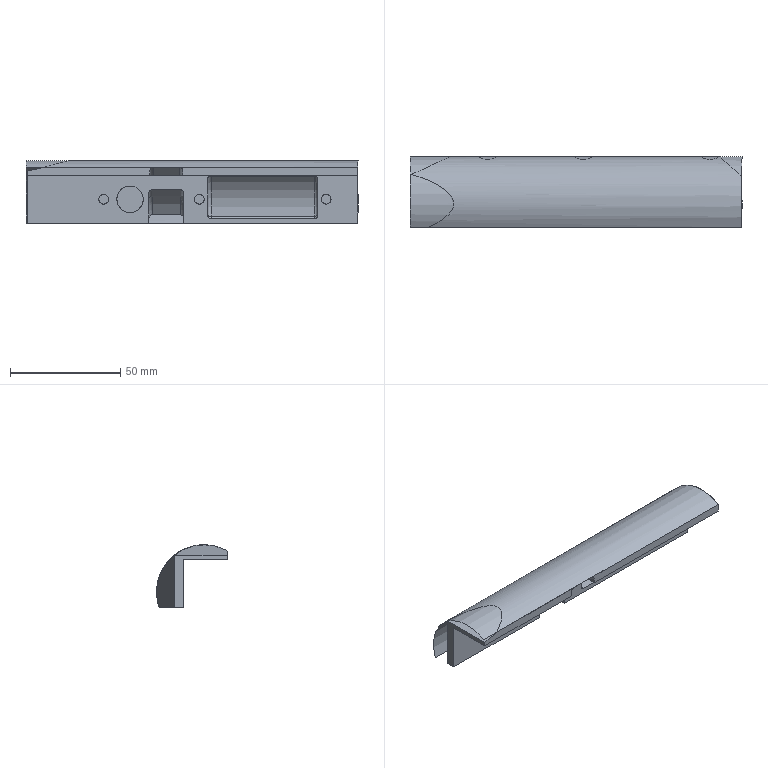NC program | Mastercam | posted with a generic post
Lines 32 to 1434 of 52802:
(10 FEM |TOOL - 9|DIA. OFF. - 9|LEN. - 9|TOOL DIA. - 10.)
N134 T9 M6
N136 G0 G54 G90 X-82.823 Y-24.256 C0. B0. S6500 M3
N138 G43 H9 Z20.
N140 Z1.
N142 G1 Z-16.25 F600.
N144 X-83.124 Y-23.448 Z-16.368 F4000.
N146 G3 X-83.642 Y-22.642 Z-16.5 I-2.109 J-.785
N148 G1 X-83.884 Y-22.278
N150 X-84.136 Y-21.786
N152 X-84.344 Y-21.317
N154 X-84.509 Y-20.881
N156 X-84.635 Y-20.477
N158 X-84.731 Y-20.104
N160 X-84.803 Y-19.761
N162 X-84.857 Y-19.444
N164 X-84.898 Y-19.15
N166 X-84.952 Y-18.629
N168 X-84.985 Y-18.155
N170 X-85.006 Y-17.715
N172 X-85.018 Y-17.3
N174 X-85.025 Y-16.902
N176 X-85.029 Y-16.516
N178 X-85.031 Y-16.138
N180 X-85.032 Y-15.766
N182 X-85.031 Y-15.397
N184 X-85.03 Y-15.031
N186 X-85.029 Y-14.667
N188 X-85.027 Y-14.303
N190 X-85.026 Y-13.94
N192 X-85.024 Y-13.577
N194 X-85.022 Y-13.215
N196 X-85.02 Y-12.852
N198 X-85.018 Y-12.49
N200 X-85.016 Y-12.127
N202 X-85.014 Y-11.765
N204 X-85.012 Y-11.402
N206 X-85.011 Y-11.04
N208 X-85.009 Y-10.677
N210 X-85.007 Y-10.314
N212 X-85.005 Y-9.951
N214 X-85.003 Y-9.588
N216 X-85.001 Y-9.226
N218 X-84.999 Y-8.863
N220 X-84.997 Y-8.5
N222 X-84.995 Y-8.137
N224 X-84.993 Y-7.774
N226 X-84.991 Y-7.41
N228 X-84.989 Y-7.047
N230 X-84.988 Y-6.684
N232 X-84.986 Y-6.321
N234 X-84.984 Y-5.958
N236 X-84.982 Y-5.594
N238 X-84.98 Y-5.231
N240 X-84.978 Y-4.867
N242 X-84.976 Y-4.504
N244 X-84.974 Y-4.14
N246 X-84.972 Y-3.777
N248 X-84.97 Y-3.413
N250 X-84.968 Y-3.05
N252 X-84.966 Y-2.686
N254 X-84.964 Y-2.322
N256 X-84.962 Y-1.958
N258 X-84.961 Y-1.595
N260 X-84.959 Y-1.231
N262 X-84.957 Y-.867
N264 X-84.955 Y-.503
N266 X-84.953 Y-.139
N268 X-84.951 Y.225
N270 X-84.949 Y.589
N272 X-84.947 Y.953
N274 X-84.945 Y1.317
N276 X-84.943 Y1.681
N278 X-84.941 Y2.045
N280 X-84.939 Y2.409
N282 X-84.937 Y2.773
N284 X-84.935 Y3.138
N286 X-84.934 Y3.502
N288 X-84.932 Y3.866
N290 X-84.93 Y4.23
N292 X-84.928 Y4.595
N294 X-84.926 Y4.959
N296 X-84.924 Y5.323
N298 X-84.922 Y5.688
N300 X-84.92 Y6.052
N302 X-84.918 Y6.417
N304 X-84.916 Y6.781
N306 X-84.914 Y7.146
N308 X-84.912 Y7.51
N310 X-84.91 Y7.875
N312 X-84.908 Y8.24
N314 X-84.906 Y8.604
N316 X-84.905 Y8.969
N318 X-84.903 Y9.333
N320 X-84.901 Y9.698
N322 X-84.899 Y10.063
N324 X-84.897 Y10.428
N326 X-84.895 Y10.792
N328 X-84.893 Y11.157
N330 X-84.891 Y11.522
N332 X-84.889 Y11.887
N334 X-84.887 Y12.252
N336 X-84.885 Y12.617
N338 X-84.883 Y12.982
N340 X-84.881 Y13.346
N342 X-84.879 Y13.711
N344 X-84.877 Y14.076
N346 X-84.876 Y14.441
N348 X-84.874 Y14.806
N350 X-84.872 Y15.171
N352 X-84.87 Y15.537
N354 X-84.868 Y15.902
N356 X-84.866 Y16.267
N358 X-84.864 Y16.632
N360 X-84.862 Y16.997
N362 X-84.86 Y17.374
N364 X-84.843 Y17.804
N366 X-84.784 Y18.268
N368 X-84.68 Y18.729
N370 X-84.532 Y19.182
N372 X-84.344 Y19.62
N374 X-84.12 Y20.036
N376 X-83.865 Y20.427
N378 X-83.585 Y20.789
N380 X-83.287 Y21.121
N382 X-82.974 Y21.423
N384 X-82.653 Y21.695
N386 X-82.326 Y21.938
N388 X-81.999 Y22.154
N390 X-81.672 Y22.346
N392 X-81.349 Y22.515
N394 X-81.032 Y22.664
N396 X-80.721 Y22.794
N398 X-80.417 Y22.909
N400 X-80.12 Y23.009
N402 X-79.831 Y23.096
N404 X-79.55 Y23.173
N406 X-79.019 Y23.298
N408 X-78.513 Y23.395
N410 X-78.027 Y23.471
N412 X-77.561 Y23.53
N414 X-77.111 Y23.577
N416 X-76.675 Y23.614
N418 X-76.251 Y23.642
N420 X-75.838 Y23.665
N422 X-75.433 Y23.683
N424 X-75.035 Y23.697
N426 X-74.642 Y23.707
N428 X-74.255 Y23.715
N430 X-73.872 Y23.722
N432 X-73.491 Y23.726
N434 X-73.114 Y23.729
N436 X-72.739 Y23.732
N438 X-72.366 Y23.733
N440 X-71.994
N442 X-71.623
N444 X-71.254
N446 X-70.885 Y23.732
N448 X-70.517 Y23.731
N450 X-70.149 Y23.73
N452 X-69.782 Y23.728
N454 X-69.415 Y23.727
N456 X-69.048 Y23.725
N458 X-68.682 Y23.723
N460 X-68.315 Y23.722
N462 X-67.948 Y23.72
N464 X-67.582 Y23.718
N466 X-67.216 Y23.716
N468 X-66.849 Y23.714
N470 X-66.483 Y23.712
N472 X-66.116 Y23.71
N474 X-65.75 Y23.708
N476 X-65.384 Y23.707
N478 X-65.017 Y23.705
N480 X-64.651 Y23.703
N482 X-64.285 Y23.701
N484 X-63.918 Y23.699
N486 X-63.552 Y23.697
N488 X-63.186 Y23.695
N490 X-62.819 Y23.693
N492 X-62.453 Y23.691
N494 X-62.086 Y23.689
N496 X-61.72 Y23.687
N498 X-61.354 Y23.685
N500 X-60.987 Y23.683
N502 X-60.621 Y23.681
N504 X-60.254 Y23.679
N506 X-59.888 Y23.677
N508 X-59.521 Y23.676
N510 X-59.155 Y23.674
N512 X-58.788 Y23.672
N514 X-58.422 Y23.67
N516 X-58.055 Y23.668
N518 X-57.689 Y23.666
N520 X-57.322 Y23.664
N522 X-56.956 Y23.662
N524 X-56.589 Y23.66
N526 X-56.221 Y23.658
N528 X-55.853 Y23.657
N530 X-55.485 Y23.656
N532 X-55.116 Y23.655
N534 X-54.747 Y23.654
N536 X-54.378
N538 X-54.008 Y23.653
N540 X-53.638
N542 X-53.269 Y23.652
N544 X-52.899
N546 X-52.529
N548 X-52.158 Y23.651
N550 X-51.788
N552 X-51.418
N554 X-51.048
N556 X-50.677
N558 X-50.307
N560 X-49.936 Y23.65
N562 X-49.566
N564 X-49.195
N566 X-48.825
N568 X-48.454
N570 X-48.084
N572 X-47.713
N574 X-47.343
N576 X-46.972
N578 X-46.602
N580 X-46.231
N582 X-45.861
N584 X-45.49
N586 X-45.119
N588 X-44.749
N590 X-44.378
N592 X-44.008
N594 X-43.637
N596 X-43.266
N598 X-42.896
N600 X-42.525
N602 X-42.155
N604 X-41.784
N606 X-41.413
N608 X-41.043
N610 X-40.672
N612 X-40.302
N614 X-39.931
N616 X-39.56
N618 X-39.19
N620 X-38.819
N622 X-38.449
N624 X-38.078
N626 X-37.707
N628 X-37.337
N630 X-36.966
N632 X-36.596
N634 X-36.225
N636 X-35.854
N638 X-35.484
N640 X-35.113
N642 X-34.743
N644 X-34.372
N646 X-34.001
N648 X-33.631
N650 X-33.26
N652 X-32.89
N654 X-32.519
N656 X-32.148
N658 X-31.778
N660 X-31.407
N662 X-31.037
N664 X-30.666
N666 X-30.295
N668 X-29.925
N670 X-29.554
N672 X-29.184
N674 X-28.813
N676 X-28.442
N678 X-28.072
N680 X-27.701
N682 X-27.331
N684 X-26.96
N686 X-26.589
N688 X-26.219
N690 X-25.848
N692 X-25.477
N694 X-25.107
N696 X-24.736
N698 X-24.366
N700 X-23.995
N702 X-23.624
N704 X-23.254
N706 X-22.883
N708 X-22.513
N710 X-22.142
N712 X-21.771
N714 X-21.401
N716 X-21.03
N718 X-20.66
N720 X-20.289
N722 X-19.918
N724 X-19.548
N726 X-19.177
N728 X-18.807
N730 X-18.436
N732 X-18.065
N734 X-17.695
N736 X-17.324
N738 X-16.954
N740 X-16.583
N742 X-16.212
N744 X-15.842
N746 X-15.471
N748 X-15.101
N750 X-14.73
N752 X-14.359
N754 X-13.989
N756 X-13.618
N758 X-13.248
N760 X-12.877
N762 X-12.506
N764 X-12.136
N766 X-11.765
N768 X-11.395
N770 X-11.024
N772 X-10.653
N774 X-10.283
N776 X-9.912
N778 X-9.542
N780 X-9.171
N782 X-8.8
N784 X-8.43
N786 X-8.059
N788 X-7.689
N790 X-7.318
N792 X-6.947
N794 X-6.577
N796 X-6.206
N798 X-5.835
N800 X-5.465
N802 X-5.094
N804 X-4.724
N806 X-4.353
N808 X-3.982
N810 X-3.612
N812 X-3.241
N814 X-2.871
N816 X-2.5
N818 X-2.129
N820 X-1.759
N822 X-1.388
N824 X-1.018
N826 X-.647
N828 X-.276
N830 X.094
N832 X.465
N834 X.835
N836 X1.206
N838 X1.577
N840 X1.947
N842 X2.318
N844 X2.688
N846 X3.059
N848 X3.43
N850 X3.8
N852 X4.171
N854 X4.541
N856 X4.912
N858 X5.283
N860 X5.653
N862 X6.024
N864 X6.394
N866 X6.765
N868 X7.136
N870 X7.506
N872 X7.877
N874 X8.247
N876 X8.618
N878 X8.989
N880 X9.359
N882 X9.73
N884 X10.1
N886 X10.471
N888 X10.842
N890 X11.212
N892 X11.583
N894 X11.953
N896 X12.324
N898 X12.695
N900 X13.065
N902 X13.436
N904 X13.807
N906 X14.177
N908 X14.548
N910 X14.918
N912 X15.289
N914 X15.66
N916 X16.03
N918 X16.401
N920 X16.771
N922 X17.142
N924 X17.513
N926 X17.883
N928 X18.254
N930 X18.624
N932 X18.995
N934 X19.366
N936 X19.736
N938 X20.107
N940 X20.477
N942 X20.848
N944 X21.219
N946 X21.589
N948 X21.96
N950 X22.33
N952 X22.701
N954 X23.072
N956 X23.442
N958 X23.813
N960 X24.183
N962 X24.554
N964 X24.925
N966 X25.295
N968 X25.666
N970 X26.036
N972 X26.407
N974 X26.778
N976 X27.148
N978 X27.519
N980 X27.889
N982 X28.26
N984 X28.631
N986 X29.001
N988 X29.372
N990 X29.742
N992 X30.113
N994 X30.484
N996 X30.854
N998 X31.225
N1000 X31.596
N1002 X31.966
N1004 X32.337
N1006 X32.707
N1008 X33.078
N1010 X33.449
N1012 X33.819
N1014 X34.19
N1016 X34.56
N1018 X34.931
N1020 X35.302
N1022 X35.672
N1024 X36.043
N1026 X36.413
N1028 X36.784
N1030 X37.155
N1032 X37.525
N1034 X37.896
N1036 X38.266
N1038 X38.637
N1040 X39.008
N1042 X39.378
N1044 X39.749
N1046 X40.119
N1048 X40.49
N1050 X40.861
N1052 X41.231
N1054 X41.602
N1056 X41.972
N1058 X42.343
N1060 X42.714
N1062 X43.084
N1064 X43.455
N1066 X43.825
N1068 X44.196
N1070 X44.567
N1072 X44.937
N1074 X45.308
N1076 X45.678
N1078 X46.049
N1080 X46.42
N1082 X46.79
N1084 X47.161
N1086 X47.531
N1088 X47.902
N1090 X48.273
N1092 X48.643
N1094 X49.014
N1096 X49.384
N1098 X49.755
N1100 X50.126
N1102 X50.496
N1104 X50.867
N1106 X51.238
N1108 X51.608
N1110 X51.979
N1112 X52.349
N1114 X52.72
N1116 X53.091
N1118 X53.461
N1120 X53.832
N1122 X54.202
N1124 X54.573
N1126 X54.944
N1128 X55.314
N1130 X55.685
N1132 X56.055
N1134 X56.426
N1136 X56.797
N1138 X57.167
N1140 X57.538
N1142 X57.908
N1144 X58.279
N1146 X58.65
N1148 X59.02
N1150 X59.391
N1152 X59.761
N1154 X60.132
N1156 X60.503
N1158 X60.873
N1160 X61.244
N1162 X61.614
N1164 X61.985
N1166 X62.356
N1168 X62.726
N1170 X63.097
N1172 X63.467
N1174 X63.838
N1176 X64.209
N1178 X64.579
N1180 X64.95
N1182 X65.32
N1184 X65.691
N1186 X66.062
N1188 X66.432
N1190 X66.803
N1192 X67.173
N1194 X67.544
N1196 X67.915
N1198 X68.285
N1200 X68.656
N1202 X69.026
N1204 X69.397
N1206 X69.768
N1208 X70.138
N1210 X70.509
N1212 X70.88
N1214 X71.25
N1216 X71.621
N1218 X71.991
N1220 X72.362
N1222 X72.733
N1224 X73.103
N1226 X73.474
N1228 X73.844
N1230 X74.215
N1232 X74.586
N1234 X74.956
N1236 X75.327
N1238 X75.697
N1240 X76.068
N1242 X76.439
N1244 X76.809
N1246 X77.18
N1248 X77.55
N1250 X77.971 Y23.649
N1252 X78.348 Y23.632
N1254 X78.718 Y23.587
N1256 X79.092 Y23.512
N1258 X79.466 Y23.406
N1260 X79.836 Y23.27
N1262 X80.197 Y23.107
N1264 X80.546 Y22.919
N1266 X80.88 Y22.707
N1268 X81.198 Y22.476
N1270 X81.497 Y22.227
N1272 X81.777 Y21.965
N1274 X82.037 Y21.692
N1276 X82.277 Y21.41
N1278 X82.498 Y21.123
N1280 X82.701 Y20.832
N1282 X82.885 Y20.539
N1284 X83.053 Y20.247
N1286 X83.206 Y19.955
N1288 X83.344 Y19.665
N1290 X83.468 Y19.379
N1292 X83.581 Y19.096
N1294 X83.683 Y18.817
N1296 X83.774 Y18.542
N1298 X83.929 Y18.016
N1300 X84.056 Y17.507
N1302 X84.159 Y17.013
N1304 X84.244 Y16.535
N1306 X84.313 Y16.071
N1308 X84.37 Y15.62
N1310 X84.417 Y15.18
N1312 X84.456 Y14.75
N1314 X84.488 Y14.328
N1316 X84.514 Y13.914
N1318 X84.536 Y13.506
N1320 X84.555 Y13.104
N1322 X84.57 Y12.707
N1324 X84.583 Y12.314
N1326 X84.594 Y11.924
N1328 X84.603 Y11.537
N1330 X84.61 Y11.153
N1332 X84.617 Y10.771
N1334 X84.622 Y10.39
N1336 X84.626 Y10.012
N1338 X84.63 Y9.634
N1340 X84.633 Y9.258
N1342 X84.636 Y8.882
N1344 X84.638 Y8.507
N1346 X84.64 Y8.133
N1348 X84.642 Y7.759
N1350 X84.643 Y7.386
N1352 X84.644 Y7.013
N1354 X84.645 Y6.641
N1356 X84.646 Y6.269
N1358 Y5.897
N1360 X84.647 Y5.525
N1362 Y5.154
N1364 X84.648 Y4.783
N1366 Y4.411
N1368 Y4.04
N1370 X84.649 Y3.669
N1372 Y3.298
N1374 Y2.927
N1376 Y2.556
N1378 Y2.185
N1380 Y1.815
N1382 X84.65 Y1.444
N1384 Y1.073
N1386 Y.702
N1388 Y.332
N1390 Y-.039
N1392 Y-.41
N1394 Y-.78
N1396 Y-1.151
N1398 Y-1.522
N1400 Y-1.892
N1402 Y-2.263
N1404 Y-2.634
N1406 Y-3.004
N1408 Y-3.375
N1410 Y-3.745
N1412 Y-4.116
N1414 Y-4.487
N1416 Y-4.857
N1418 Y-5.228
N1420 Y-5.599
N1422 Y-5.969
N1424 Y-6.34
N1426 Y-6.71
N1428 Y-7.081
N1430 Y-7.452
N1432 Y-7.822
N1434 Y-8.193
N1436 Y-8.563
N1438 Y-8.934
N1440 Y-9.305
N1442 Y-9.675
N1444 Y-10.046
N1446 Y-10.416
N1448 Y-10.787
N1450 Y-11.158
N1452 Y-11.528
N1454 Y-11.899
N1456 Y-12.269
N1458 Y-12.64
N1460 Y-13.011
N1462 Y-13.381
N1464 Y-13.752
N1466 Y-14.122
N1468 Y-14.493
N1470 Y-14.864
N1472 Y-15.234
N1474 Y-15.605
N1476 Y-15.976
N1478 Y-16.346
N1480 Y-16.717
N1482 Y-16.939
N1484 X84.635 Y-17.315
N1486 X84.592 Y-17.684
N1488 X84.52 Y-18.058
N1490 X84.416 Y-18.432
N1492 X84.284 Y-18.802
N1494 X84.123 Y-19.164
N1496 X83.937 Y-19.515
N1498 X83.727 Y-19.851
N1500 X83.497 Y-20.17
N1502 X83.25 Y-20.471
N1504 X82.989 Y-20.752
N1506 X82.717 Y-21.014
N1508 X82.436 Y-21.256
N1510 X82.149 Y-21.479
N1512 X81.859 Y-21.683
N1514 X81.566 Y-21.869
N1516 X81.273 Y-22.039
N1518 X80.981 Y-22.192
N1520 X80.691 Y-22.332
N1522 X80.405 Y-22.458
N1524 X80.121 Y-22.571
N1526 X79.842 Y-22.674
N1528 X79.567 Y-22.766
N1530 X79.04 Y-22.923
N1532 X78.53 Y-23.05
N1534 X78.036 Y-23.155
N1536 X77.557 Y-23.24
N1538 X77.092 Y-23.31
N1540 X76.64 Y-23.368
N1542 X76.2 Y-23.415
N1544 X75.769 Y-23.454
N1546 X75.347 Y-23.486
N1548 X74.933 Y-23.513
N1550 X74.525 Y-23.536
N1552 X74.123 Y-23.554
N1554 X73.725 Y-23.57
N1556 X73.332 Y-23.582
N1558 X72.942 Y-23.593
N1560 X72.555 Y-23.602
N1562 X72.171 Y-23.61
N1564 X71.789 Y-23.616
N1566 X71.408 Y-23.622
N1568 X71.029 Y-23.626
N1570 X70.651 Y-23.63
N1572 X70.275 Y-23.633
N1574 X69.899 Y-23.636
N1576 X69.524 Y-23.638
N1578 X69.15 Y-23.64
N1580 X68.777 Y-23.641
N1582 X68.403 Y-23.643
N1584 X68.031 Y-23.644
N1586 X67.658 Y-23.645
N1588 X67.286 Y-23.646
N1590 X66.914
N1592 X66.543 Y-23.647
N1594 X66.171
N1596 X65.8 Y-23.648
N1598 X65.428
N1600 X65.057
N1602 X64.686 Y-23.649
N1604 X64.315
N1606 X63.944
N1608 X63.573
N1610 X63.203
N1612 X62.832
N1614 X62.461 Y-23.65
N1616 X62.09
N1618 X61.72
N1620 X61.349
N1622 X60.978
N1624 X60.607
N1626 X60.237
N1628 X59.866
N1630 X59.495
N1632 X59.125
N1634 X58.754
N1636 X58.384
N1638 X58.013
N1640 X57.642
N1642 X57.272
N1644 X56.901
N1646 X56.53
N1648 X56.16
N1650 X55.789
N1652 X55.419
N1654 X55.048
N1656 X54.677
N1658 X54.307
N1660 X53.936
N1662 X53.566
N1664 X53.195
N1666 X52.824
N1668 X52.454
N1670 X52.083
N1672 X51.713
N1674 X51.342
N1676 X50.971
N1678 X50.601
N1680 X50.23
N1682 X49.86
N1684 X49.489
N1686 X49.118
N1688 X48.748
N1690 X48.377
N1692 X48.006
N1694 X47.636
N1696 X47.265
N1698 X46.895
N1700 X46.524
N1702 X46.153
N1704 X45.783
N1706 X45.412
N1708 X45.042
N1710 X44.671
N1712 X44.3
N1714 X43.93
N1716 X43.559
N1718 X43.189
N1720 X42.818
N1722 X42.447
N1724 X42.077
N1726 X41.706
N1728 X41.336
N1730 X40.965
N1732 X40.594
N1734 X40.224
N1736 X39.853
N1738 X39.483
N1740 X39.112
N1742 X38.741
N1744 X38.371
N1746 X38.
N1748 X37.63
N1750 X37.259
N1752 X36.888
N1754 X36.518
N1756 X36.147
N1758 X35.777
N1760 X35.406
N1762 X35.035
N1764 X34.665
N1766 X34.294
N1768 X33.924
N1770 X33.553
N1772 X33.182
N1774 X32.812
N1776 X32.441
N1778 X32.071
N1780 X31.7
N1782 X31.329
N1784 X30.959
N1786 X30.588
N1788 X30.217
N1790 X29.847
N1792 X29.476
N1794 X29.106
N1796 X28.735
N1798 X28.364
N1800 X27.994
N1802 X27.623
N1804 X27.253
N1806 X26.882
N1808 X26.511
N1810 X26.141
N1812 X25.77
N1814 X25.4
N1816 X25.029
N1818 X24.658
N1820 X24.288
N1822 X23.917
N1824 X23.547
N1826 X23.176
N1828 X22.805
N1830 X22.435
N1832 X22.064
N1834 X21.694
N1836 X21.323
N1838 X20.952
N1840 X20.582
N1842 X20.211
N1844 X19.841
N1846 X19.47
N1848 X19.099
N1850 X18.729
N1852 X18.358
N1854 X17.988
N1856 X17.617
N1858 X17.246
N1860 X16.876
N1862 X16.505
N1864 X16.135
N1866 X15.764
N1868 X15.393
N1870 X15.023
N1872 X14.652
N1874 X14.282
N1876 X13.911
N1878 X13.54
N1880 X13.17
N1882 X12.799
N1884 X12.429
N1886 X12.058
N1888 X11.687
N1890 X11.317
N1892 X10.946
N1894 X10.575
N1896 X10.205
N1898 X9.834
N1900 X9.464
N1902 X9.093
N1904 X8.722
N1906 X8.352
N1908 X7.981
N1910 X7.611
N1912 X7.24
N1914 X6.869
N1916 X6.499
N1918 X6.128
N1920 X5.758
N1922 X5.387
N1924 X5.016
N1926 X4.646
N1928 X4.275
N1930 X3.905
N1932 X3.534
N1934 X3.163
N1936 X2.793
N1938 X2.422
N1940 X2.052
N1942 X1.681
N1944 X1.31
N1946 X.94
N1948 X.569
N1950 X.199
N1952 X-.172
N1954 X-.543
N1956 X-.913
N1958 X-1.284
N1960 X-1.654
N1962 X-2.025
N1964 X-2.396
N1966 X-2.766
N1968 X-3.137
N1970 X-3.507
N1972 X-3.878
N1974 X-4.249
N1976 X-4.619
N1978 X-4.99
N1980 X-5.36
N1982 X-5.731
N1984 X-6.102
N1986 X-6.472
N1988 X-6.843
N1990 X-7.213
N1992 X-7.584
N1994 X-7.955
N1996 X-8.325
N1998 X-8.696
N2000 X-9.067
N2002 X-9.437
N2004 X-9.808
N2006 X-10.178
N2008 X-10.549
N2010 X-10.92
N2012 X-11.29
N2014 X-11.661
N2016 X-12.031
N2018 X-12.402
N2020 X-12.773
N2022 X-13.143
N2024 X-13.514
N2026 X-13.884
N2028 X-14.255
N2030 X-14.626
N2032 X-14.996
N2034 X-15.367
N2036 X-15.737
N2038 X-16.108
N2040 X-16.479
N2042 X-16.849
N2044 X-17.22
N2046 X-17.59
N2048 X-17.961
N2050 X-18.332
N2052 X-18.702
N2054 X-19.073
N2056 X-19.443
N2058 X-19.814
N2060 X-20.185
N2062 X-20.555
N2064 X-20.926
N2066 X-21.296
N2068 X-21.667
N2070 X-22.038
N2072 X-22.408
N2074 X-22.779
N2076 X-23.149
N2078 X-23.52
N2080 X-23.891
N2082 X-24.261
N2084 X-24.632
N2086 X-25.002
N2088 X-25.373
N2090 X-25.744
N2092 X-26.114
N2094 X-26.485
N2096 X-26.855
N2098 X-27.226
N2100 X-27.597
N2102 X-27.967
N2104 X-28.338
N2106 X-28.709
N2108 X-29.079
N2110 X-29.45
N2112 X-29.82
N2114 X-30.191
N2116 X-30.562
N2118 X-30.932
N2120 X-31.303
N2122 X-31.673
N2124 X-32.044
N2126 X-32.415
N2128 X-32.785
N2130 X-33.156
N2132 X-33.526
N2134 X-33.897
N2136 X-34.268
N2138 X-34.638
N2140 X-35.009
N2142 X-35.379
N2144 X-35.75
N2146 X-36.121
N2148 X-36.491
N2150 X-36.862
N2152 X-37.232
N2154 X-37.603
N2156 X-37.974
N2158 X-38.344
N2160 X-38.715
N2162 X-39.085
N2164 X-39.456
N2166 X-39.827
N2168 X-40.197
N2170 X-40.568
N2172 X-40.938
N2174 X-41.309
N2176 X-41.68
N2178 X-42.05
N2180 X-42.421
N2182 X-42.791
N2184 X-43.162
N2186 X-43.533
N2188 X-43.903
N2190 X-44.274
N2192 X-44.644
N2194 X-45.015
N2196 X-45.386
N2198 X-45.756
N2200 X-46.127
N2202 X-46.497
N2204 X-46.868
N2206 X-47.239
N2208 X-47.609
N2210 X-47.98
N2212 X-48.351
N2214 X-48.721
N2216 X-49.092
N2218 X-49.462
N2220 X-49.833
N2222 X-50.204
N2224 X-50.574
N2226 X-50.945
N2228 X-51.315
N2230 X-51.686
N2232 X-52.057
N2234 X-52.427
N2236 X-52.798
N2238 X-53.168
N2240 X-53.539
N2242 X-53.91
N2244 X-54.28
N2246 X-54.651
N2248 X-55.021
N2250 X-55.392
N2252 X-55.763
N2254 X-56.133
N2256 X-56.504
N2258 X-56.874
N2260 X-57.245
N2262 X-57.616
N2264 X-57.986
N2266 X-58.357
N2268 X-58.727
N2270 X-59.098
N2272 X-59.469
N2274 X-59.839
N2276 X-60.21
N2278 X-60.58
N2280 X-60.951
N2282 X-61.322
N2284 X-61.692
N2286 X-62.063
N2288 X-62.433
N2290 X-62.804
N2292 X-63.175
N2294 X-63.545
N2296 X-63.916
N2298 X-64.286
N2300 X-64.657
N2302 X-65.028
N2304 X-65.398
N2306 X-65.769
N2308 X-66.139
N2310 X-66.51
N2312 X-66.881
N2314 X-67.251
N2316 X-67.622
N2318 X-67.993
N2320 X-68.363
N2322 X-68.734
N2324 X-69.104
N2326 X-69.475
N2328 X-69.846
N2330 X-70.216
N2332 X-70.587
N2334 X-70.957
N2336 X-71.328
N2338 X-71.699
N2340 X-72.069
N2342 X-72.44
N2344 X-72.81
N2346 X-73.181
N2348 X-73.552
N2350 X-73.922
N2352 X-74.293
N2354 X-74.663
N2356 X-75.034
N2358 X-75.405
N2360 X-75.775
N2362 X-76.146
N2364 X-76.516
N2366 X-76.887
N2368 X-77.258
N2370 X-77.628
N2372 X-78.014 Y-23.636
N2374 X-78.404 Y-23.593
N2376 X-78.79 Y-23.52
N2378 X-79.172 Y-23.418
N2380 X-79.546 Y-23.289
N2382 X-79.911 Y-23.133
N2384 X-80.264 Y-22.953
N2386 X-80.603 Y-22.75
N2388 X-80.925 Y-22.528
N2390 X-81.23 Y-22.288
N2392 X-81.517 Y-22.033
N2394 X-81.784 Y-21.767
N2396 X-82.033 Y-21.491
N2398 X-82.262 Y-21.208
N2400 X-82.473 Y-20.92
N2402 X-82.667 Y-20.63
N2404 X-82.843 Y-20.337
N2406 X-83.004 Y-20.046
N2408 X-83.149 Y-19.755
N2410 X-83.282 Y-19.466
N2412 X-83.401 Y-19.181
N2414 X-83.509 Y-18.899
N2416 X-83.606 Y-18.622
N2418 X-83.694 Y-18.348
N2420 X-83.842 Y-17.824
N2422 X-83.962 Y-17.316
N2424 X-84.061 Y-16.825
N2426 X-84.141 Y-16.348
N2428 X-84.206 Y-15.885
N2430 X-84.259 Y-15.435
N2432 X-84.303 Y-14.996
N2434 X-84.339 Y-14.567
N2436 X-84.368 Y-14.146
N2438 X-84.392 Y-13.732
N2440 X-84.411 Y-13.325
N2442 X-84.427 Y-12.924
N2444 X-84.44 Y-12.527
N2446 X-84.451 Y-12.134
N2448 X-84.459 Y-11.745
N2450 X-84.466 Y-11.358
N2452 X-84.471 Y-10.974
N2454 X-84.475 Y-10.592
N2456 X-84.479 Y-10.212
N2458 X-84.481 Y-9.833
N2460 X-84.483 Y-9.456
N2462 X-84.484 Y-9.079
N2464 Y-8.704
N2466 X-84.485 Y-8.329
N2468 X-84.484 Y-7.955
N2470 Y-7.581
N2472 X-84.483 Y-7.208
N2474 X-84.482 Y-6.836
N2476 X-84.481 Y-6.463
N2478 X-84.48 Y-6.091
N2480 X-84.479 Y-5.719
N2482 X-84.477 Y-5.348
N2484 X-84.476 Y-4.976
N2486 X-84.474 Y-4.605
N2488 X-84.473 Y-4.234
N2490 X-84.471 Y-3.862
N2492 X-84.469 Y-3.491
N2494 X-84.468 Y-3.12
N2496 X-84.466 Y-2.749
N2498 X-84.464 Y-2.379
N2500 X-84.462 Y-2.008
N2502 X-84.46 Y-1.637
N2504 X-84.458 Y-1.266
N2506 X-84.456 Y-.895
N2508 X-84.455 Y-.525
N2510 X-84.453 Y-.154
N2512 X-84.451 Y.217
N2514 X-84.449 Y.587
N2516 X-84.447 Y.958
N2518 X-84.445 Y1.329
N2520 X-84.443 Y1.699
N2522 X-84.441 Y2.07
N2524 X-84.439 Y2.441
N2526 X-84.437 Y2.811
N2528 X-84.435 Y3.182
N2530 X-84.433 Y3.552
N2532 X-84.431 Y3.923
N2534 X-84.429 Y4.294
N2536 X-84.427 Y4.664
N2538 X-84.425 Y5.035
N2540 X-84.423 Y5.406
N2542 X-84.421 Y5.776
N2544 X-84.419 Y6.147
N2546 X-84.417 Y6.517
N2548 X-84.416 Y6.888
N2550 X-84.414 Y7.259
N2552 X-84.412 Y7.629
N2554 X-84.41 Y8.
N2556 X-84.408 Y8.37
N2558 X-84.406 Y8.741
N2560 X-84.404 Y9.112
N2562 X-84.402 Y9.482
N2564 X-84.4 Y9.853
N2566 X-84.398 Y10.223
N2568 X-84.396 Y10.594
N2570 X-84.394 Y10.965
N2572 X-84.392 Y11.335
N2574 X-84.39 Y11.706
N2576 X-84.388 Y12.076
N2578 X-84.386 Y12.447
N2580 X-84.384 Y12.818
N2582 X-84.382 Y13.188
N2584 X-84.38 Y13.559
N2586 X-84.378 Y13.929
N2588 X-84.376 Y14.3
N2590 X-84.374 Y14.671
N2592 X-84.372 Y15.041
N2594 X-84.365 Y15.54
N2596 X-84.341 Y15.902
N2598 X-84.298 Y16.273
N2600 X-84.233 Y16.647
N2602 X-84.146 Y17.019
N2604 X-84.038 Y17.387
N2606 X-83.908 Y17.747
N2608 X-83.758 Y18.097
N2610 X-83.59 Y18.437
N2612 X-83.403 Y18.766
N2614 X-83.2 Y19.081
N2616 X-82.982 Y19.382
N2618 X-82.753 Y19.667
N2620 X-82.512 Y19.938
N2622 X-82.262 Y20.193
N2624 X-82.004 Y20.432
N2626 X-81.74 Y20.656
N2628 X-81.471 Y20.865
N2630 X-81.198 Y21.06
N2632 X-80.923 Y21.24
N2634 X-80.647 Y21.408
N2636 X-80.371 Y21.562
N2638 X-80.094 Y21.705
N2640 X-79.82 Y21.835
N2642 X-79.546 Y21.956
N2644 X-79.275 Y22.066
N2646 X-79.006 Y22.168
N2648 X-78.486 Y22.342
N2650 X-77.978 Y22.489
N2652 X-77.482 Y22.612
N2654 X-76.998 Y22.715
N2656 X-76.526 Y22.801
N2658 X-76.065 Y22.873
N2660 X-75.615 Y22.933
N2662 X-75.174 Y22.983
N2664 X-74.742 Y23.024
N2666 X-74.317 Y23.059
N2668 X-73.9 Y23.088
N2670 X-73.489 Y23.111
N2672 X-73.083 Y23.131
N2674 X-72.683 Y23.147
N2676 X-72.286 Y23.161
N2678 X-71.893 Y23.171
N2680 X-71.504 Y23.18
N2682 X-71.117 Y23.187
N2684 X-70.733 Y23.193
N2686 X-70.35 Y23.198
N2688 X-69.97 Y23.201
N2690 X-69.591 Y23.204
N2692 X-69.213 Y23.206
N2694 X-68.836 Y23.207
N2696 X-68.461 Y23.208
N2698 X-68.086
N2700 X-67.711
N2702 X-67.338
N2704 X-66.964 Y23.207
N2706 X-66.591
N2708 X-66.219 Y23.206
N2710 X-65.847 Y23.204
N2712 X-65.475 Y23.203
N2714 X-65.103 Y23.202
N2716 X-64.731 Y23.2
N2718 X-64.36 Y23.199
N2720 X-63.989 Y23.197
N2722 X-63.618 Y23.196
N2724 X-63.246 Y23.194
N2726 X-62.875 Y23.192
N2728 X-62.504 Y23.19
N2730 X-62.134 Y23.189
N2732 X-61.763 Y23.187
N2734 X-61.392 Y23.185
N2736 X-61.021 Y23.183
N2738 X-60.65 Y23.181
N2740 X-60.28 Y23.179
N2742 X-59.909 Y23.177
N2744 X-59.538 Y23.175
N2746 X-59.168 Y23.173
N2748 X-58.797 Y23.171
N2750 X-58.427 Y23.17
N2752 X-58.057 Y23.168
N2754 X-57.688 Y23.166
N2756 X-57.319 Y23.164
N2758 X-56.949 Y23.163
N2760 X-56.58 Y23.161
N2762 X-56.211 Y23.16
N2764 X-55.841 Y23.159
N2766 X-55.472 Y23.158
N2768 X-55.103 Y23.157
N2770 X-54.733 Y23.156
N2772 X-54.363 Y23.155
N2774 X-53.994
N2776 X-53.624 Y23.154
N2778 X-53.254
N2780 X-52.884 Y23.153
N2782 X-52.514
N2784 X-52.144 Y23.152
N2786 X-51.774
N2788 X-51.404
N2790 X-51.033
N2792 X-50.663 Y23.151
N2794 X-50.293
N2796 X-49.923
N2798 X-49.552
N2800 X-49.182
N2802 X-48.811
N2804 X-48.441
N2806 X-48.07
N2808 X-47.7 Y23.15
N2810 X-47.329
N2812 X-46.959
N2814 X-46.588
N2816 X-46.218
N2818 X-45.847
N2820 X-45.477
N2822 X-45.106
N2824 X-44.736
N2826 X-44.365
N2828 X-43.994
N2830 X-43.624
N2832 X-43.253
N2834 X-42.883
N2836 X-42.512
N2838 X-42.142
N2840 X-41.771
N2842 X-41.4
N2844 X-41.03
N2846 X-40.659
N2848 X-40.289
N2850 X-39.918
N2852 X-39.547
N2854 X-39.177
N2856 X-38.806
N2858 X-38.436
N2860 X-38.065
N2862 X-37.694
N2864 X-37.324
N2866 X-36.953
N2868 X-36.583
N2870 X-36.212
N2872 X-35.841
N2874 X-35.471
N2876 X-35.1
N2878 X-34.73
N2880 X-34.359
N2882 X-33.988
N2884 X-33.618
N2886 X-33.247
N2888 X-32.877
N2890 X-32.506
N2892 X-32.135
N2894 X-31.765
N2896 X-31.394
N2898 X-31.024
N2900 X-30.653
N2902 X-30.282
N2904 X-29.912
N2906 X-29.541
N2908 X-29.17
N2910 X-28.8
N2912 X-28.429
N2914 X-28.059
N2916 X-27.688
N2918 X-27.317
N2920 X-26.947
N2922 X-26.576
N2924 X-26.206
N2926 X-25.835
N2928 X-25.464
N2930 X-25.094
N2932 X-24.723
N2934 X-24.353
N2936 X-23.982